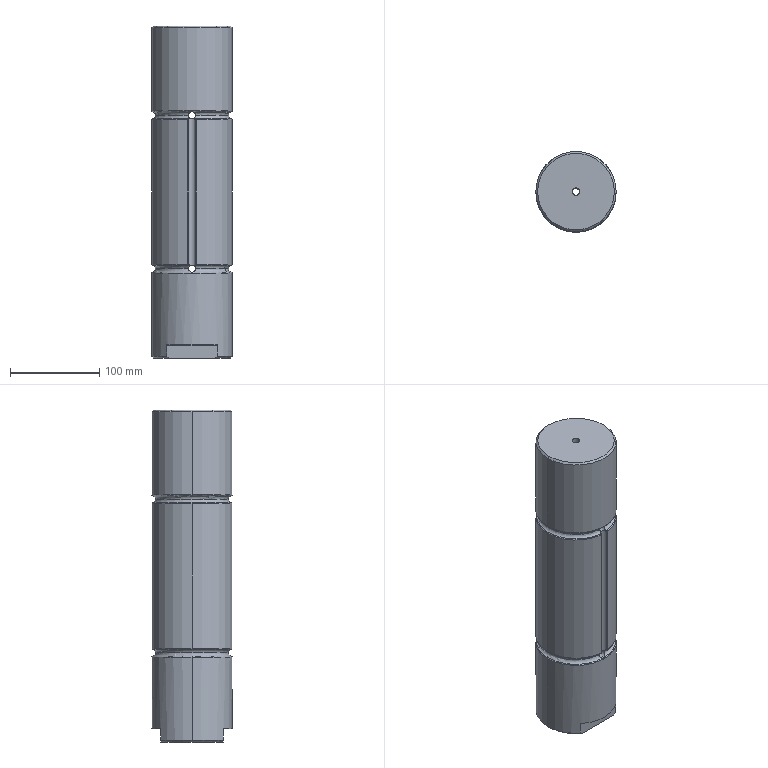Part | SolidWorks | features Fillet 5, ICE 5, 3DProfileFeature 2, HoleWzd 2, MirrorPattern 2, RevCut 2, Chamfer 1, Extrusion 1, RefAxis 1 | 1 solid | 91 faces | box 90 x 90 x 372 mm | volume 2295512 mm3 | cylinder 35 | torus 22 | cone 11 | spline 8 | sphere 8 | plane 7 | commonest cylinder face diameters 8 x16 90 x7 2 x6 8.5 x4 30 x2